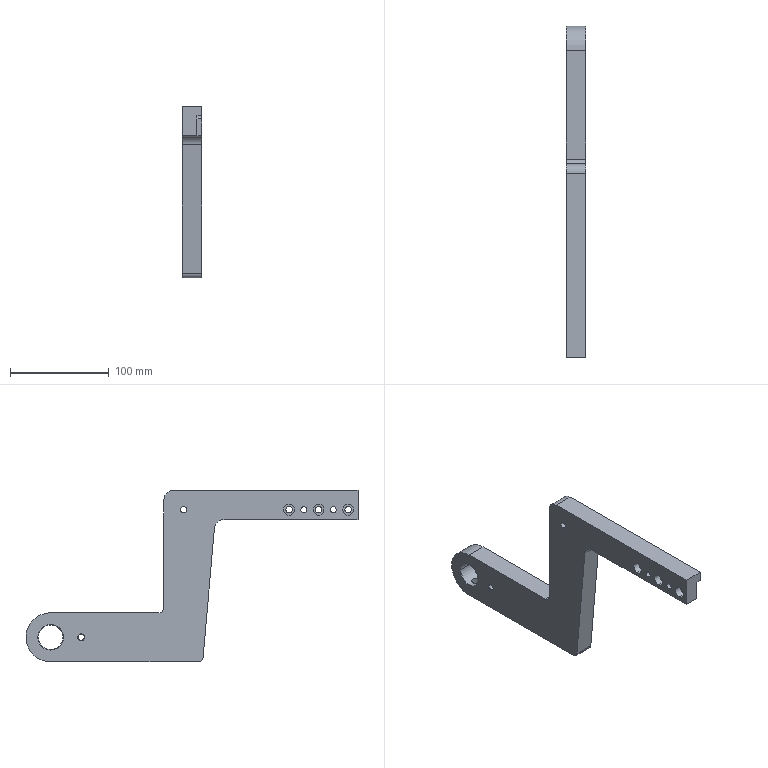Part | NX | features BREP 1 | 1 solid | 62 faces | box 20 x 337 x 174.5 mm | volume 360815 mm3 | cylinder 34 | plane 16 | cone 12 | commonest cylinder face diameters 6 x8 6.5 x8 11 x8 8.5 x2 10 x2 20 x2